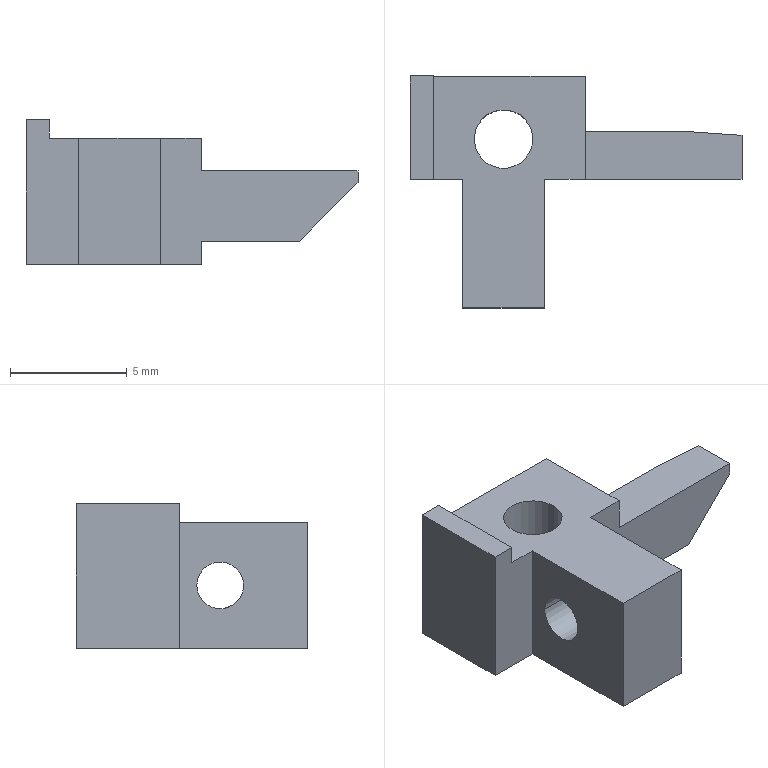Part | NX | 1 solid | 25 faces | box 14.2 x 9.913 x 6.2 mm | volume 267.475 mm3 | plane 19 | cylinder 6 | commonest cylinder face diameters 2 x2 2.5 x2 3.1 x2
STEP:
#1=CARTESIAN_POINT('',(-48.11,-45.316,4.403));
#2=VERTEX_POINT('',#1);
#3=CARTESIAN_POINT('',(-54.61,-45.316,4.403));
#4=VERTEX_POINT('',#3);
#5=CARTESIAN_POINT('',(-49.101,-45.316,4.403));
#6=DIRECTION('',(-1.,0.,0.));
#7=VECTOR('',#6,1000.);
#8=LINE('',#5,#7);
#9=EDGE_CURVE('',#2,#4,#8,.T.);
#10=ORIENTED_EDGE('',*,*,#9,.F.);
#11=CARTESIAN_POINT('',(-48.11,-45.316,-0.9969));
#12=VERTEX_POINT('',#11);
#13=CARTESIAN_POINT('',(-48.11,-45.316,4.403));
#14=DIRECTION('',(0.,0.,-1.));
#15=VECTOR('',#14,1000.);
#16=LINE('',#13,#15);
#17=EDGE_CURVE('',#2,#12,#16,.T.);
#18=ORIENTED_EDGE('',*,*,#17,.T.);
#19=CARTESIAN_POINT('',(-55.61,-45.316,-0.9969));
#20=VERTEX_POINT('',#19);
#21=CARTESIAN_POINT('',(-49.101,-45.316,-0.9969));
#22=DIRECTION('',(-1.,0.,0.));
#23=VECTOR('',#22,1000.);
#24=LINE('',#21,#23);
#25=EDGE_CURVE('',#12,#20,#24,.T.);
#26=ORIENTED_EDGE('',*,*,#25,.T.);
#27=CARTESIAN_POINT('',(-55.61,-45.316,5.203));
#28=VERTEX_POINT('',#27);
#29=CARTESIAN_POINT('',(-55.61,-45.316,4.403));
#30=DIRECTION('',(0.,0.,1.));
#31=VECTOR('',#30,1000.);
#32=LINE('',#29,#31);
#33=EDGE_CURVE('',#20,#28,#32,.T.);
#34=ORIENTED_EDGE('',*,*,#33,.T.);
#35=CARTESIAN_POINT('',(-54.61,-45.316,5.203));
#36=VERTEX_POINT('',#35);
#37=CARTESIAN_POINT('',(-54.61,-45.316,5.203));
#38=DIRECTION('',(-1.,0.,0.));
#39=VECTOR('',#38,1000.);
#40=LINE('',#37,#39);
#41=EDGE_CURVE('',#36,#28,#40,.T.);
#42=ORIENTED_EDGE('',*,*,#41,.F.);
#43=CARTESIAN_POINT('',(-54.61,-45.316,4.403));
#44=DIRECTION('',(0.,0.,1.));
#45=VECTOR('',#44,1000.);
#46=LINE('',#43,#45);
#47=EDGE_CURVE('',#4,#36,#46,.T.);
#48=ORIENTED_EDGE('',*,*,#47,.F.);
#49=EDGE_LOOP('',(#10,#18,#26,#34,#42,#48));
#50=FACE_BOUND('',#49,.T.);
#51=CARTESIAN_POINT('',(-48.11,-45.316,4.403));
#52=DIRECTION('',(0.,1.,0.));
#53=DIRECTION('',(0.,0.,-1.));
#54=AXIS2_PLACEMENT_3D('',#51,#52,#53);
#55=PLANE('',#54);
#56=ADVANCED_FACE('',(#50),#55,.T.);
#57=CARTESIAN_POINT('',(-48.11,-49.729,-0.9969));
#58=VERTEX_POINT('',#57);
#59=CARTESIAN_POINT('',(-48.11,-51.163,-0.9969));
#60=DIRECTION('',(0.,1.,0.));
#61=VECTOR('',#60,1000.);
#62=LINE('',#59,#61);
#63=EDGE_CURVE('',#58,#12,#62,.T.);
#64=ORIENTED_EDGE('',*,*,#63,.F.);
#65=CARTESIAN_POINT('',(-49.86,-49.729,-0.9969));
#66=VERTEX_POINT('',#65);
#67=CARTESIAN_POINT('',(-49.101,-49.729,-0.9969));
#68=DIRECTION('',(-1.,0.,0.));
#69=VECTOR('',#68,1000.);
#70=LINE('',#67,#69);
#71=EDGE_CURVE('',#58,#66,#70,.T.);
#72=ORIENTED_EDGE('',*,*,#71,.T.);
#73=CARTESIAN_POINT('',(-49.86,-55.229,-0.9969));
#74=VERTEX_POINT('',#73);
#75=CARTESIAN_POINT('',(-49.86,-51.163,-0.9969));
#76=DIRECTION('',(0.,-1.,0.));
#77=VECTOR('',#76,1000.);
#78=LINE('',#75,#77);
#79=EDGE_CURVE('',#66,#74,#78,.T.);
#80=ORIENTED_EDGE('',*,*,#79,.T.);
#81=CARTESIAN_POINT('',(-53.36,-55.229,-0.9969));
#82=VERTEX_POINT('',#81);
#83=CARTESIAN_POINT('',(-49.86,-55.229,-0.9969));
#84=DIRECTION('',(-1.,0.,0.));
#85=VECTOR('',#84,1000.);
#86=LINE('',#83,#85);
#87=EDGE_CURVE('',#74,#82,#86,.T.);
#88=ORIENTED_EDGE('',*,*,#87,.T.);
#89=CARTESIAN_POINT('',(-53.36,-49.729,-0.9969));
#90=VERTEX_POINT('',#89);
#91=CARTESIAN_POINT('',(-53.36,-51.163,-0.9969));
#92=DIRECTION('',(0.,-1.,0.));
#93=VECTOR('',#92,1000.);
#94=LINE('',#91,#93);
#95=EDGE_CURVE('',#90,#82,#94,.T.);
#96=ORIENTED_EDGE('',*,*,#95,.F.);
#97=CARTESIAN_POINT('',(-55.61,-49.729,-0.9969));
#98=VERTEX_POINT('',#97);
#99=CARTESIAN_POINT('',(-49.101,-49.729,-0.9969));
#100=DIRECTION('',(-1.,0.,0.));
#101=VECTOR('',#100,1000.);
#102=LINE('',#99,#101);
#103=EDGE_CURVE('',#90,#98,#102,.T.);
#104=ORIENTED_EDGE('',*,*,#103,.T.);
#105=CARTESIAN_POINT('',(-55.61,-51.163,-0.9969));
#106=DIRECTION('',(0.,1.,0.));
#107=VECTOR('',#106,1000.);
#108=LINE('',#105,#107);
#109=EDGE_CURVE('',#98,#20,#108,.T.);
#110=ORIENTED_EDGE('',*,*,#109,.T.);
#111=ORIENTED_EDGE('',*,*,#25,.F.);
#112=EDGE_LOOP('',(#64,#72,#80,#88,#96,#104,#110,#111));
#113=FACE_BOUND('',#112,.T.);
#114=CARTESIAN_POINT('',(-50.36,-48.012,-0.9969));
#115=VERTEX_POINT('',#114);
#116=CARTESIAN_POINT('',(-52.86,-48.012,-0.9969));
#117=VERTEX_POINT('',#116);
#118=CARTESIAN_POINT('',(-51.61,-48.012,-0.9969));
#119=DIRECTION('',(0.,0.,-1.));
#120=DIRECTION('',(-1.,0.,0.));
#121=AXIS2_PLACEMENT_3D('',#118,#119,#120);
#122=CIRCLE('',#121,1.25);
#123=EDGE_CURVE('',#115,#117,#122,.T.);
#124=ORIENTED_EDGE('',*,*,#123,.F.);
#125=CARTESIAN_POINT('',(-51.61,-48.012,-0.9969));
#126=DIRECTION('',(0.,0.,-1.));
#127=DIRECTION('',(-1.,0.,0.));
#128=AXIS2_PLACEMENT_3D('',#125,#126,#127);
#129=CIRCLE('',#128,1.25);
#130=EDGE_CURVE('',#117,#115,#129,.T.);
#131=ORIENTED_EDGE('',*,*,#130,.F.);
#132=EDGE_LOOP('',(#124,#131));
#133=FACE_BOUND('',#132,.T.);
#134=CARTESIAN_POINT('',(-50.06,-53.51,-0.9969));
#135=VERTEX_POINT('',#134);
#136=CARTESIAN_POINT('',(-53.16,-53.51,-0.9969));
#137=VERTEX_POINT('',#136);
#138=CARTESIAN_POINT('',(-51.61,-53.51,-0.9969));
#139=DIRECTION('',(0.,0.,-1.));
#140=DIRECTION('',(-1.,0.,0.));
#141=AXIS2_PLACEMENT_3D('',#138,#139,#140);
#142=CIRCLE('',#141,1.55);
#143=EDGE_CURVE('',#135,#137,#142,.T.);
#144=ORIENTED_EDGE('',*,*,#143,.F.);
#145=CARTESIAN_POINT('',(-51.61,-53.51,-0.9969));
#146=DIRECTION('',(0.,0.,-1.));
#147=DIRECTION('',(-1.,0.,0.));
#148=AXIS2_PLACEMENT_3D('',#145,#146,#147);
#149=CIRCLE('',#148,1.55);
#150=EDGE_CURVE('',#137,#135,#149,.T.);
#151=ORIENTED_EDGE('',*,*,#150,.F.);
#152=EDGE_LOOP('',(#144,#151));
#153=FACE_BOUND('',#152,.T.);
#154=CARTESIAN_POINT('',(-49.101,-51.163,-0.9969));
#155=DIRECTION('',(0.,0.,-1.));
#156=DIRECTION('',(0.,-1.,0.));
#157=AXIS2_PLACEMENT_3D('',#154,#155,#156);
#158=PLANE('',#157);
#159=ADVANCED_FACE('',(#113,#133,#153),#158,.T.);
#160=ORIENTED_EDGE('',*,*,#63,.T.);
#161=ORIENTED_EDGE('',*,*,#17,.F.);
#162=CARTESIAN_POINT('',(-48.11,-49.729,4.403));
#163=VERTEX_POINT('',#162);
#164=CARTESIAN_POINT('',(-48.11,-51.163,4.403));
#165=DIRECTION('',(0.,1.,0.));
#166=VECTOR('',#165,1000.);
#167=LINE('',#164,#166);
#168=EDGE_CURVE('',#163,#2,#167,.T.);
#169=ORIENTED_EDGE('',*,*,#168,.F.);
#170=CARTESIAN_POINT('',(-48.11,-49.729,3.003));
#171=VERTEX_POINT('',#170);
#172=CARTESIAN_POINT('',(-48.11,-49.729,4.403));
#173=DIRECTION('',(0.,0.,-1.));
#174=VECTOR('',#173,1000.);
#175=LINE('',#172,#174);
#176=EDGE_CURVE('',#163,#171,#175,.T.);
#177=ORIENTED_EDGE('',*,*,#176,.T.);
#178=CARTESIAN_POINT('',(-48.11,-47.687,3.003));
#179=VERTEX_POINT('',#178);
#180=CARTESIAN_POINT('',(-48.11,-51.163,3.003));
#181=DIRECTION('',(0.,-1.,0.));
#182=VECTOR('',#181,1000.);
#183=LINE('',#180,#182);
#184=EDGE_CURVE('',#179,#171,#183,.T.);
#185=ORIENTED_EDGE('',*,*,#184,.F.);
#186=CARTESIAN_POINT('',(-48.11,-47.687,0.003122));
#187=VERTEX_POINT('',#186);
#188=CARTESIAN_POINT('',(-48.11,-47.687,4.403));
#189=DIRECTION('',(0.,0.,1.));
#190=VECTOR('',#189,1000.);
#191=LINE('',#188,#190);
#192=EDGE_CURVE('',#187,#179,#191,.T.);
#193=ORIENTED_EDGE('',*,*,#192,.F.);
#194=CARTESIAN_POINT('',(-48.11,-49.729,0.003122));
#195=VERTEX_POINT('',#194);
#196=CARTESIAN_POINT('',(-48.11,-51.163,0.003122));
#197=DIRECTION('',(0.,1.,0.));
#198=VECTOR('',#197,1000.);
#199=LINE('',#196,#198);
#200=EDGE_CURVE('',#195,#187,#199,.T.);
#201=ORIENTED_EDGE('',*,*,#200,.F.);
#202=CARTESIAN_POINT('',(-48.11,-49.729,4.403));
#203=DIRECTION('',(0.,0.,-1.));
#204=VECTOR('',#203,1000.);
#205=LINE('',#202,#204);
#206=EDGE_CURVE('',#195,#58,#205,.T.);
#207=ORIENTED_EDGE('',*,*,#206,.T.);
#208=EDGE_LOOP('',(#160,#161,#169,#177,#185,#193,#201,#207));
#209=FACE_BOUND('',#208,.T.);
#210=CARTESIAN_POINT('',(-48.11,-47.529,-0.5969));
#211=DIRECTION('',(1.,0.,0.));
#212=DIRECTION('',(0.,1.,0.));
#213=AXIS2_PLACEMENT_3D('',#210,#211,#212);
#214=PLANE('',#213);
#215=ADVANCED_FACE('',(#209),#214,.T.);
#216=CARTESIAN_POINT('',(-55.61,-49.729,5.203));
#217=VERTEX_POINT('',#216);
#218=CARTESIAN_POINT('',(-55.61,-45.316,5.203));
#219=DIRECTION('',(0.,-1.,0.));
#220=VECTOR('',#219,1000.);
#221=LINE('',#218,#220);
#222=EDGE_CURVE('',#28,#217,#221,.T.);
#223=ORIENTED_EDGE('',*,*,#222,.T.);
#224=CARTESIAN_POINT('',(-54.61,-49.729,5.203));
#225=VERTEX_POINT('',#224);
#226=CARTESIAN_POINT('',(-55.61,-49.729,5.203));
#227=DIRECTION('',(1.,0.,0.));
#228=VECTOR('',#227,1000.);
#229=LINE('',#226,#228);
#230=EDGE_CURVE('',#217,#225,#229,.T.);
#231=ORIENTED_EDGE('',*,*,#230,.T.);
#232=CARTESIAN_POINT('',(-54.61,-49.729,5.203));
#233=DIRECTION('',(0.,1.,0.));
#234=VECTOR('',#233,1000.);
#235=LINE('',#232,#234);
#236=EDGE_CURVE('',#225,#36,#235,.T.);
#237=ORIENTED_EDGE('',*,*,#236,.T.);
#238=ORIENTED_EDGE('',*,*,#41,.T.);
#239=EDGE_LOOP('',(#223,#231,#237,#238));
#240=FACE_BOUND('',#239,.T.);
#241=CARTESIAN_POINT('',(-55.143,-49.311,5.203));
#242=DIRECTION('',(0.,0.,1.));
#243=DIRECTION('',(1.,0.,0.));
#244=AXIS2_PLACEMENT_3D('',#241,#242,#243);
#245=PLANE('',#244);
#246=ADVANCED_FACE('',(#240),#245,.T.);
#247=CARTESIAN_POINT('',(-55.61,-49.729,4.403));
#248=DIRECTION('',(0.,0.,-1.));
#249=VECTOR('',#248,1000.);
#250=LINE('',#247,#249);
#251=EDGE_CURVE('',#217,#98,#250,.T.);
#252=ORIENTED_EDGE('',*,*,#251,.F.);
#253=ORIENTED_EDGE('',*,*,#222,.F.);
#254=ORIENTED_EDGE('',*,*,#33,.F.);
#255=ORIENTED_EDGE('',*,*,#109,.F.);
#256=EDGE_LOOP('',(#252,#253,#254,#255));
#257=FACE_BOUND('',#256,.T.);
#258=CARTESIAN_POINT('',(-55.61,-49.729,4.403));
#259=DIRECTION('',(-1.,0.,0.));
#260=DIRECTION('',(0.,0.,1.));
#261=AXIS2_PLACEMENT_3D('',#258,#259,#260);
#262=PLANE('',#261);
#263=ADVANCED_FACE('',(#257),#262,.T.);
#264=CARTESIAN_POINT('',(-54.61,-49.729,4.403));
#265=VERTEX_POINT('',#264);
#266=CARTESIAN_POINT('',(-54.61,-51.163,4.403));
#267=DIRECTION('',(0.,-1.,0.));
#268=VECTOR('',#267,1000.);
#269=LINE('',#266,#268);
#270=EDGE_CURVE('',#4,#265,#269,.T.);
#271=ORIENTED_EDGE('',*,*,#270,.F.);
#272=ORIENTED_EDGE('',*,*,#47,.T.);
#273=ORIENTED_EDGE('',*,*,#236,.F.);
#274=CARTESIAN_POINT('',(-54.61,-49.729,4.403));
#275=DIRECTION('',(0.,0.,1.));
#276=VECTOR('',#275,1000.);
#277=LINE('',#274,#276);
#278=EDGE_CURVE('',#265,#225,#277,.T.);
#279=ORIENTED_EDGE('',*,*,#278,.F.);
#280=EDGE_LOOP('',(#271,#272,#273,#279));
#281=FACE_BOUND('',#280,.T.);
#282=CARTESIAN_POINT('',(-54.61,-45.316,4.403));
#283=DIRECTION('',(1.,0.,0.));
#284=DIRECTION('',(0.,1.,0.));
#285=AXIS2_PLACEMENT_3D('',#282,#283,#284);
#286=PLANE('',#285);
#287=ADVANCED_FACE('',(#281),#286,.T.);
#288=ORIENTED_EDGE('',*,*,#278,.T.);
#289=ORIENTED_EDGE('',*,*,#230,.F.);
#290=ORIENTED_EDGE('',*,*,#251,.T.);
#291=ORIENTED_EDGE('',*,*,#103,.F.);
#292=CARTESIAN_POINT('',(-53.36,-49.729,4.403));
#293=VERTEX_POINT('',#292);
#294=CARTESIAN_POINT('',(-53.36,-49.729,4.403));
#295=DIRECTION('',(0.,0.,1.));
#296=VECTOR('',#295,1000.);
#297=LINE('',#294,#296);
#298=EDGE_CURVE('',#90,#293,#297,.T.);
#299=ORIENTED_EDGE('',*,*,#298,.T.);
#300=CARTESIAN_POINT('',(-49.101,-49.729,4.403));
#301=DIRECTION('',(1.,0.,0.));
#302=VECTOR('',#301,1000.);
#303=LINE('',#300,#302);
#304=EDGE_CURVE('',#265,#293,#303,.T.);
#305=ORIENTED_EDGE('',*,*,#304,.F.);
#306=EDGE_LOOP('',(#288,#289,#290,#291,#299,#305));
#307=FACE_BOUND('',#306,.T.);
#308=CARTESIAN_POINT('',(-54.61,-49.729,4.403));
#309=DIRECTION('',(0.,-1.,0.));
#310=DIRECTION('',(0.,0.,-1.));
#311=AXIS2_PLACEMENT_3D('',#308,#309,#310);
#312=PLANE('',#311);
#313=ADVANCED_FACE('',(#307),#312,.T.);
#314=CARTESIAN_POINT('',(-43.739,-47.687,3.003));
#315=VERTEX_POINT('',#314);
#316=CARTESIAN_POINT('',(-49.101,-47.687,3.003));
#317=DIRECTION('',(1.,0.,0.));
#318=VECTOR('',#317,1000.);
#319=LINE('',#316,#318);
#320=EDGE_CURVE('',#179,#315,#319,.T.);
#321=ORIENTED_EDGE('',*,*,#320,.F.);
#322=ORIENTED_EDGE('',*,*,#184,.T.);
#323=CARTESIAN_POINT('',(-41.41,-49.729,3.003));
#324=VERTEX_POINT('',#323);
#325=CARTESIAN_POINT('',(-49.101,-49.729,3.003));
#326=DIRECTION('',(1.,0.,0.));
#327=VECTOR('',#326,1000.);
#328=LINE('',#325,#327);
#329=EDGE_CURVE('',#171,#324,#328,.T.);
#330=ORIENTED_EDGE('',*,*,#329,.T.);
#331=CARTESIAN_POINT('',(-41.41,-47.851,3.003));
#332=VERTEX_POINT('',#331);
#333=CARTESIAN_POINT('',(-41.41,-51.163,3.003));
#334=DIRECTION('',(0.,1.,0.));
#335=VECTOR('',#334,1000.);
#336=LINE('',#333,#335);
#337=EDGE_CURVE('',#324,#332,#336,.T.);
#338=ORIENTED_EDGE('',*,*,#337,.T.);
#339=CARTESIAN_POINT('',(-49.101,-47.307,3.003));
#340=DIRECTION('',(0.9975,-0.07053,0.));
#341=VECTOR('',#340,1000.);
#342=LINE('',#339,#341);
#343=EDGE_CURVE('',#315,#332,#342,.T.);
#344=ORIENTED_EDGE('',*,*,#343,.F.);
#345=EDGE_LOOP('',(#321,#322,#330,#338,#344));
#346=FACE_BOUND('',#345,.T.);
#347=CARTESIAN_POINT('',(-48.11,-53.629,3.003));
#348=DIRECTION('',(0.,0.,1.));
#349=DIRECTION('',(1.,0.,0.));
#350=AXIS2_PLACEMENT_3D('',#347,#348,#349);
#351=PLANE('',#350);
#352=ADVANCED_FACE('',(#346),#351,.T.);
#353=ORIENTED_EDGE('',*,*,#123,.T.);
#354=CARTESIAN_POINT('',(-52.86,-48.012,4.403));
#355=VERTEX_POINT('',#354);
#356=CARTESIAN_POINT('',(-52.86,-48.012,-2.597));
#357=DIRECTION('',(0.,0.,-1.));
#358=VECTOR('',#357,1000.);
#359=LINE('',#356,#358);
#360=EDGE_CURVE('',#117,#355,#359,.F.);
#361=ORIENTED_EDGE('',*,*,#360,.T.);
#362=CARTESIAN_POINT('',(-50.36,-48.012,4.403));
#363=VERTEX_POINT('',#362);
#364=CARTESIAN_POINT('',(-51.61,-48.012,4.403));
#365=DIRECTION('',(0.,0.,-1.));
#366=DIRECTION('',(-1.,0.,0.));
#367=AXIS2_PLACEMENT_3D('',#364,#365,#366);
#368=CIRCLE('',#367,1.25);
#369=EDGE_CURVE('',#363,#355,#368,.T.);
#370=ORIENTED_EDGE('',*,*,#369,.F.);
#371=CARTESIAN_POINT('',(-50.36,-48.012,-2.597));
#372=DIRECTION('',(0.,0.,-1.));
#373=VECTOR('',#372,1000.);
#374=LINE('',#371,#373);
#375=EDGE_CURVE('',#115,#363,#374,.F.);
#376=ORIENTED_EDGE('',*,*,#375,.F.);
#377=EDGE_LOOP('',(#353,#361,#370,#376));
#378=FACE_BOUND('',#377,.T.);
#379=CARTESIAN_POINT('',(-51.61,-48.012,-2.597));
#380=DIRECTION('',(0.,0.,-1.));
#381=DIRECTION('',(-1.,0.,0.));
#382=AXIS2_PLACEMENT_3D('',#379,#380,#381);
#383=CYLINDRICAL_SURFACE('',#382,1.25);
#384=ADVANCED_FACE('',(#378),#383,.F.);
#385=ORIENTED_EDGE('',*,*,#320,.T.);
#386=CARTESIAN_POINT('',(-46.739,-47.687,0.003122));
#387=VERTEX_POINT('',#386);
#388=CARTESIAN_POINT('',(-44.574,-47.687,2.167));
#389=DIRECTION('',(0.7071,0.,0.7071));
#390=VECTOR('',#389,1000.);
#391=LINE('',#388,#390);
#392=EDGE_CURVE('',#387,#315,#391,.T.);
#393=ORIENTED_EDGE('',*,*,#392,.F.);
#394=CARTESIAN_POINT('',(-49.101,-47.687,0.003122));
#395=DIRECTION('',(-1.,0.,0.));
#396=VECTOR('',#395,1000.);
#397=LINE('',#394,#396);
#398=EDGE_CURVE('',#387,#187,#397,.T.);
#399=ORIENTED_EDGE('',*,*,#398,.T.);
#400=ORIENTED_EDGE('',*,*,#192,.T.);
#401=EDGE_LOOP('',(#385,#393,#399,#400));
#402=FACE_BOUND('',#401,.T.);
#403=CARTESIAN_POINT('',(-48.11,-47.687,2.503));
#404=DIRECTION('',(0.,1.,0.));
#405=DIRECTION('',(1.,0.,0.));
#406=AXIS2_PLACEMENT_3D('',#403,#404,#405);
#407=PLANE('',#406);
#408=ADVANCED_FACE('',(#402),#407,.T.);
#409=ORIENTED_EDGE('',*,*,#143,.T.);
#410=CARTESIAN_POINT('',(-53.16,-53.51,1.003));
#411=VERTEX_POINT('',#410);
#412=CARTESIAN_POINT('',(-53.16,-53.51,-0.9969));
#413=DIRECTION('',(0.,0.,-1.));
#414=VECTOR('',#413,1000.);
#415=LINE('',#412,#414);
#416=EDGE_CURVE('',#137,#411,#415,.F.);
#417=ORIENTED_EDGE('',*,*,#416,.T.);
#418=CARTESIAN_POINT('',(-50.06,-53.51,1.003));
#419=VERTEX_POINT('',#418);
#420=CARTESIAN_POINT('',(-51.61,-53.51,1.003));
#421=DIRECTION('',(0.,0.,-1.));
#422=DIRECTION('',(-1.,0.,0.));
#423=AXIS2_PLACEMENT_3D('',#420,#421,#422);
#424=CIRCLE('',#423,1.55);
#425=EDGE_CURVE('',#419,#411,#424,.T.);
#426=ORIENTED_EDGE('',*,*,#425,.F.);
#427=CARTESIAN_POINT('',(-50.06,-53.51,-0.9969));
#428=DIRECTION('',(0.,0.,-1.));
#429=VECTOR('',#428,1000.);
#430=LINE('',#427,#429);
#431=EDGE_CURVE('',#135,#419,#430,.F.);
#432=ORIENTED_EDGE('',*,*,#431,.F.);
#433=EDGE_LOOP('',(#409,#417,#426,#432));
#434=FACE_BOUND('',#433,.T.);
#435=CARTESIAN_POINT('',(-51.61,-53.51,-0.9969));
#436=DIRECTION('',(0.,0.,-1.));
#437=DIRECTION('',(-1.,0.,0.));
#438=AXIS2_PLACEMENT_3D('',#435,#436,#437);
#439=CYLINDRICAL_SURFACE('',#438,1.55);
#440=ADVANCED_FACE('',(#434),#439,.F.);
#441=CARTESIAN_POINT('',(-41.41,-49.729,2.503));
#442=VERTEX_POINT('',#441);
#443=CARTESIAN_POINT('',(-41.41,-47.887,2.503));
#444=VERTEX_POINT('',#443);
#445=CARTESIAN_POINT('',(-41.41,-51.163,2.503));
#446=DIRECTION('',(0.,1.,0.));
#447=VECTOR('',#446,1000.);
#448=LINE('',#445,#447);
#449=EDGE_CURVE('',#442,#444,#448,.T.);
#450=ORIENTED_EDGE('',*,*,#449,.T.);
#451=CARTESIAN_POINT('',(-41.41,-47.752,4.403));
#452=DIRECTION('',(0.,-0.07053,-0.9975));
#453=VECTOR('',#452,1000.);
#454=LINE('',#451,#453);
#455=EDGE_CURVE('',#332,#444,#454,.T.);
#456=ORIENTED_EDGE('',*,*,#455,.F.);
#457=ORIENTED_EDGE('',*,*,#337,.F.);
#458=CARTESIAN_POINT('',(-41.41,-49.729,4.403));
#459=DIRECTION('',(0.,0.,-1.));
#460=VECTOR('',#459,1000.);
#461=LINE('',#458,#460);
#462=EDGE_CURVE('',#324,#442,#461,.T.);
#463=ORIENTED_EDGE('',*,*,#462,.T.);
#464=EDGE_LOOP('',(#450,#456,#457,#463));
#465=FACE_BOUND('',#464,.T.);
#466=CARTESIAN_POINT('',(-41.41,-49.37,2.047));
#467=DIRECTION('',(1.,0.,0.));
#468=DIRECTION('',(0.,1.,0.));
#469=AXIS2_PLACEMENT_3D('',#466,#467,#468);
#470=PLANE('',#469);
#471=ADVANCED_FACE('',(#465),#470,.T.);
#472=CARTESIAN_POINT('',(-43.91,-47.887,0.003122));
#473=VERTEX_POINT('',#472);
#474=CARTESIAN_POINT('',(-43.16,-47.887,0.7531));
#475=DIRECTION('',(0.7071,0.,0.7071));
#476=VECTOR('',#475,1000.);
#477=LINE('',#474,#476);
#478=EDGE_CURVE('',#473,#444,#477,.T.);
#479=ORIENTED_EDGE('',*,*,#478,.T.);
#480=ORIENTED_EDGE('',*,*,#449,.F.);
#481=CARTESIAN_POINT('',(-43.91,-49.729,0.003122));
#482=VERTEX_POINT('',#481);
#483=CARTESIAN_POINT('',(-39.51,-49.729,4.403));
#484=DIRECTION('',(-0.7071,0.,-0.7071));
#485=VECTOR('',#484,1000.);
#486=LINE('',#483,#485);
#487=EDGE_CURVE('',#442,#482,#486,.T.);
#488=ORIENTED_EDGE('',*,*,#487,.T.);
#489=CARTESIAN_POINT('',(-43.91,-51.163,0.003122));
#490=DIRECTION('',(0.,1.,0.));
#491=VECTOR('',#490,1000.);
#492=LINE('',#489,#491);
#493=EDGE_CURVE('',#482,#473,#492,.T.);
#494=ORIENTED_EDGE('',*,*,#493,.T.);
#495=EDGE_LOOP('',(#479,#480,#488,#494));
#496=FACE_BOUND('',#495,.T.);
#497=CARTESIAN_POINT('',(-43.16,-50.658,0.7531));
#498=DIRECTION('',(0.7071,0.,-0.7071));
#499=DIRECTION('',(0.,-1.,0.));
#500=AXIS2_PLACEMENT_3D('',#497,#498,#499);
#501=PLANE('',#500);
#502=ADVANCED_FACE('',(#496),#501,.T.);
#503=ORIENTED_EDGE('',*,*,#478,.F.);
#504=CARTESIAN_POINT('',(-49.101,-47.52,0.003122));
#505=DIRECTION('',(-0.9975,0.07053,0.));
#506=VECTOR('',#505,1000.);
#507=LINE('',#504,#506);
#508=EDGE_CURVE('',#473,#387,#507,.T.);
#509=ORIENTED_EDGE('',*,*,#508,.T.);
#510=ORIENTED_EDGE('',*,*,#392,.T.);
#511=ORIENTED_EDGE('',*,*,#343,.T.);
#512=ORIENTED_EDGE('',*,*,#455,.T.);
#513=EDGE_LOOP('',(#503,#509,#510,#511,#512));
#514=FACE_BOUND('',#513,.T.);
#515=CARTESIAN_POINT('',(-43.867,-47.787,1.46));
#516=DIRECTION('',(0.07036,0.995,-0.07036));
#517=DIRECTION('',(-0.7071,0.,-0.7071));
#518=AXIS2_PLACEMENT_3D('',#515,#516,#517);
#519=PLANE('',#518);
#520=ADVANCED_FACE('',(#514),#519,.T.);
#521=CARTESIAN_POINT('',(-49.101,-49.729,0.003122));
#522=DIRECTION('',(-1.,0.,0.));
#523=VECTOR('',#522,1000.);
#524=LINE('',#521,#523);
#525=EDGE_CURVE('',#482,#195,#524,.T.);
#526=ORIENTED_EDGE('',*,*,#525,.T.);
#527=ORIENTED_EDGE('',*,*,#200,.T.);
#528=ORIENTED_EDGE('',*,*,#398,.F.);
#529=ORIENTED_EDGE('',*,*,#508,.F.);
#530=ORIENTED_EDGE('',*,*,#493,.F.);
#531=EDGE_LOOP('',(#526,#527,#528,#529,#530));
#532=FACE_BOUND('',#531,.T.);
#533=CARTESIAN_POINT('',(-46.061,-49.047,0.003122));
#534=DIRECTION('',(0.,0.,-1.));
#535=DIRECTION('',(0.,-1.,0.));
#536=AXIS2_PLACEMENT_3D('',#533,#534,#535);
#537=PLANE('',#536);
#538=ADVANCED_FACE('',(#532),#537,.T.);
#539=CARTESIAN_POINT('',(-49.86,-49.729,4.403));
#540=VERTEX_POINT('',#539);
#541=CARTESIAN_POINT('',(-49.86,-49.729,4.403));
#542=DIRECTION('',(0.,0.,-1.));
#543=VECTOR('',#542,1000.);
#544=LINE('',#541,#543);
#545=EDGE_CURVE('',#540,#66,#544,.T.);
#546=ORIENTED_EDGE('',*,*,#545,.T.);
#547=ORIENTED_EDGE('',*,*,#71,.F.);
#548=ORIENTED_EDGE('',*,*,#206,.F.);
#549=ORIENTED_EDGE('',*,*,#525,.F.);
#550=ORIENTED_EDGE('',*,*,#487,.F.);
#551=ORIENTED_EDGE('',*,*,#462,.F.);
#552=ORIENTED_EDGE('',*,*,#329,.F.);
#553=ORIENTED_EDGE('',*,*,#176,.F.);
#554=CARTESIAN_POINT('',(-49.101,-49.729,4.403));
#555=DIRECTION('',(1.,0.,0.));
#556=VECTOR('',#555,1000.);
#557=LINE('',#554,#556);
#558=EDGE_CURVE('',#540,#163,#557,.T.);
#559=ORIENTED_EDGE('',*,*,#558,.F.);
#560=EDGE_LOOP('',(#546,#547,#548,#549,#550,#551,#552,#553,#559));
#561=FACE_BOUND('',#560,.T.);
#562=CARTESIAN_POINT('',(-48.11,-49.729,-0.5969));
#563=DIRECTION('',(0.,-1.,0.));
#564=DIRECTION('',(0.,0.,-1.));
#565=AXIS2_PLACEMENT_3D('',#562,#563,#564);
#566=PLANE('',#565);
#567=ADVANCED_FACE('',(#561),#566,.T.);
#568=ORIENTED_EDGE('',*,*,#298,.F.);
#569=ORIENTED_EDGE('',*,*,#95,.T.);
#570=CARTESIAN_POINT('',(-53.36,-55.229,4.403));
#571=VERTEX_POINT('',#570);
#572=CARTESIAN_POINT('',(-53.36,-55.229,4.403));
#573=DIRECTION('',(0.,0.,1.));
#574=VECTOR('',#573,1000.);
#575=LINE('',#572,#574);
#576=EDGE_CURVE('',#82,#571,#575,.T.);
#577=ORIENTED_EDGE('',*,*,#576,.T.);
#578=CARTESIAN_POINT('',(-53.36,-51.163,4.403));
#579=DIRECTION('',(0.,-1.,0.));
#580=VECTOR('',#579,1000.);
#581=LINE('',#578,#580);
#582=EDGE_CURVE('',#293,#571,#581,.T.);
#583=ORIENTED_EDGE('',*,*,#582,.F.);
#584=EDGE_LOOP('',(#568,#569,#577,#583));
#585=FACE_BOUND('',#584,.T.);
#586=CARTESIAN_POINT('',(-53.36,-50.479,1.703));
#587=VERTEX_POINT('',#586);
#588=CARTESIAN_POINT('',(-53.36,-52.479,1.703));
#589=VERTEX_POINT('',#588);
#590=CARTESIAN_POINT('',(-53.36,-51.479,1.703));
#591=DIRECTION('',(-1.,0.,0.));
#592=DIRECTION('',(0.,-1.,0.));
#593=AXIS2_PLACEMENT_3D('',#590,#591,#592);
#594=CIRCLE('',#593,1.);
#595=EDGE_CURVE('',#587,#589,#594,.T.);
#596=ORIENTED_EDGE('',*,*,#595,.F.);
#597=CARTESIAN_POINT('',(-53.36,-51.479,1.703));
#598=DIRECTION('',(-1.,0.,0.));
#599=DIRECTION('',(0.,-1.,0.));
#600=AXIS2_PLACEMENT_3D('',#597,#598,#599);
#601=CIRCLE('',#600,1.);
#602=EDGE_CURVE('',#589,#587,#601,.T.);
#603=ORIENTED_EDGE('',*,*,#602,.F.);
#604=EDGE_LOOP('',(#596,#603));
#605=FACE_BOUND('',#604,.T.);
#606=CARTESIAN_POINT('',(-53.36,-50.229,-0.9969));
#607=DIRECTION('',(-1.,0.,0.));
#608=DIRECTION('',(0.,0.,1.));
#609=AXIS2_PLACEMENT_3D('',#606,#607,#608);
#610=PLANE('',#609);
#611=ADVANCED_FACE('',(#585,#605),#610,.T.);
#612=ORIENTED_EDGE('',*,*,#545,.F.);
#613=CARTESIAN_POINT('',(-49.86,-55.229,4.403));
#614=VERTEX_POINT('',#613);
#615=CARTESIAN_POINT('',(-49.86,-51.163,4.403));
#616=DIRECTION('',(0.,1.,0.));
#617=VECTOR('',#616,1000.);
#618=LINE('',#615,#617);
#619=EDGE_CURVE('',#614,#540,#618,.T.);
#620=ORIENTED_EDGE('',*,*,#619,.F.);
#621=CARTESIAN_POINT('',(-49.86,-55.229,4.403));
#622=DIRECTION('',(0.,0.,-1.));
#623=VECTOR('',#622,1000.);
#624=LINE('',#621,#623);
#625=EDGE_CURVE('',#614,#74,#624,.T.);
#626=ORIENTED_EDGE('',*,*,#625,.T.);
#627=ORIENTED_EDGE('',*,*,#79,.F.);
#628=EDGE_LOOP('',(#612,#620,#626,#627));
#629=FACE_BOUND('',#628,.T.);
#630=CARTESIAN_POINT('',(-49.86,-50.479,1.703));
#631=VERTEX_POINT('',#630);
#632=CARTESIAN_POINT('',(-49.86,-52.479,1.703));
#633=VERTEX_POINT('',#632);
#634=CARTESIAN_POINT('',(-49.86,-51.479,1.703));
#635=DIRECTION('',(-1.,0.,0.));
#636=DIRECTION('',(0.,-1.,0.));
#637=AXIS2_PLACEMENT_3D('',#634,#635,#636);
#638=CIRCLE('',#637,1.);
#639=EDGE_CURVE('',#631,#633,#638,.T.);
#640=ORIENTED_EDGE('',*,*,#639,.T.);
#641=CARTESIAN_POINT('',(-49.86,-51.479,1.703));
#642=DIRECTION('',(-1.,0.,0.));
#643=DIRECTION('',(0.,-1.,0.));
#644=AXIS2_PLACEMENT_3D('',#641,#642,#643);
#645=CIRCLE('',#644,1.);
#646=EDGE_CURVE('',#633,#631,#645,.T.);
#647=ORIENTED_EDGE('',*,*,#646,.T.);
#648=EDGE_LOOP('',(#640,#647));
#649=FACE_BOUND('',#648,.T.);
#650=CARTESIAN_POINT('',(-49.86,-50.229,4.403));
#651=DIRECTION('',(1.,0.,0.));
#652=DIRECTION('',(0.,1.,0.));
#653=AXIS2_PLACEMENT_3D('',#650,#651,#652);
#654=PLANE('',#653);
#655=ADVANCED_FACE('',(#629,#649),#654,.T.);
#656=ORIENTED_EDGE('',*,*,#576,.F.);
#657=ORIENTED_EDGE('',*,*,#87,.F.);
#658=ORIENTED_EDGE('',*,*,#625,.F.);
#659=CARTESIAN_POINT('',(-49.101,-55.229,4.403));
#660=DIRECTION('',(1.,0.,0.));
#661=VECTOR('',#660,1000.);
#662=LINE('',#659,#661);
#663=EDGE_CURVE('',#571,#614,#662,.T.);
#664=ORIENTED_EDGE('',*,*,#663,.F.);
#665=EDGE_LOOP('',(#656,#657,#658,#664));
#666=FACE_BOUND('',#665,.T.);
#667=CARTESIAN_POINT('',(-51.674,-55.229,-0.05073));
#668=DIRECTION('',(0.,-1.,0.));
#669=DIRECTION('',(0.,0.,-1.));
#670=AXIS2_PLACEMENT_3D('',#667,#668,#669);
#671=PLANE('',#670);
#672=ADVANCED_FACE('',(#666),#671,.T.);
#673=ORIENTED_EDGE('',*,*,#639,.F.);
#674=CARTESIAN_POINT('',(-40.04,-50.479,1.703));
#675=DIRECTION('',(-1.,0.,0.));
#676=VECTOR('',#675,1000.);
#677=LINE('',#674,#676);
#678=EDGE_CURVE('',#587,#631,#677,.F.);
#679=ORIENTED_EDGE('',*,*,#678,.F.);
#680=ORIENTED_EDGE('',*,*,#595,.T.);
#681=CARTESIAN_POINT('',(-40.04,-52.479,1.703));
#682=DIRECTION('',(-1.,0.,0.));
#683=VECTOR('',#682,1000.);
#684=LINE('',#681,#683);
#685=EDGE_CURVE('',#589,#633,#684,.F.);
#686=ORIENTED_EDGE('',*,*,#685,.T.);
#687=EDGE_LOOP('',(#673,#679,#680,#686));
#688=FACE_BOUND('',#687,.T.);
#689=CARTESIAN_POINT('',(-52.427,-52.193,1.003));
#690=VERTEX_POINT('',#689);
#691=CARTESIAN_POINT('',(-50.793,-52.193,1.003));
#692=VERTEX_POINT('',#691);
#693=CARTESIAN_POINT('',(-52.427,-52.193,1.003));
#694=CARTESIAN_POINT('',(-52.414,-52.185,0.9943));
#695=CARTESIAN_POINT('',(-52.399,-52.176,0.986));
#696=CARTESIAN_POINT('',(-52.385,-52.168,0.9781));
#697=CARTESIAN_POINT('',(-52.37,-52.159,0.9701));
#698=CARTESIAN_POINT('',(-52.356,-52.151,0.9626));
#699=CARTESIAN_POINT('',(-52.341,-52.143,0.9555));
#700=CARTESIAN_POINT('',(-52.326,-52.135,0.9484));
#701=CARTESIAN_POINT('',(-52.311,-52.127,0.9417));
#702=CARTESIAN_POINT('',(-52.295,-52.12,0.9353));
#703=CARTESIAN_POINT('',(-52.28,-52.112,0.929));
#704=CARTESIAN_POINT('',(-52.264,-52.105,0.923));
#705=CARTESIAN_POINT('',(-52.248,-52.097,0.9173));
#706=CARTESIAN_POINT('',(-52.232,-52.09,0.9116));
#707=CARTESIAN_POINT('',(-52.215,-52.083,0.9062));
#708=CARTESIAN_POINT('',(-52.199,-52.076,0.9012));
#709=CARTESIAN_POINT('',(-52.183,-52.07,0.8962));
#710=CARTESIAN_POINT('',(-52.166,-52.063,0.8914));
#711=CARTESIAN_POINT('',(-52.149,-52.057,0.887));
#712=CARTESIAN_POINT('',(-52.132,-52.051,0.8826));
#713=CARTESIAN_POINT('',(-52.115,-52.045,0.8785));
#714=CARTESIAN_POINT('',(-52.098,-52.039,0.8746));
#715=CARTESIAN_POINT('',(-52.081,-52.033,0.8708));
#716=CARTESIAN_POINT('',(-52.063,-52.028,0.8672));
#717=CARTESIAN_POINT('',(-52.046,-52.023,0.8639));
#718=CARTESIAN_POINT('',(-52.029,-52.018,0.8606));
#719=CARTESIAN_POINT('',(-52.011,-52.013,0.8575));
#720=CARTESIAN_POINT('',(-51.993,-52.008,0.8547));
#721=CARTESIAN_POINT('',(-51.976,-52.004,0.8519));
#722=CARTESIAN_POINT('',(-51.958,-52.,0.8494));
#723=CARTESIAN_POINT('',(-51.94,-51.996,0.847));
#724=CARTESIAN_POINT('',(-51.905,-51.988,0.8423));
#725=CARTESIAN_POINT('',(-51.868,-51.981,0.8385));
#726=CARTESIAN_POINT('',(-51.832,-51.976,0.8355));
#727=CARTESIAN_POINT('',(-51.795,-51.971,0.8324));
#728=CARTESIAN_POINT('',(-51.758,-51.967,0.8302));
#729=CARTESIAN_POINT('',(-51.721,-51.964,0.8287));
#730=CARTESIAN_POINT('',(-51.685,-51.962,0.8273));
#731=CARTESIAN_POINT('',(-51.647,-51.96,0.8265));
#732=CARTESIAN_POINT('',(-51.61,-51.96,0.8265));
#733=CARTESIAN_POINT('',(-51.573,-51.96,0.8265));
#734=CARTESIAN_POINT('',(-51.536,-51.962,0.8273));
#735=CARTESIAN_POINT('',(-51.5,-51.964,0.8287));
#736=CARTESIAN_POINT('',(-51.481,-51.965,0.8294));
#737=CARTESIAN_POINT('',(-51.463,-51.967,0.8304));
#738=CARTESIAN_POINT('',(-51.445,-51.969,0.8315));
#739=CARTESIAN_POINT('',(-51.427,-51.971,0.8326));
#740=CARTESIAN_POINT('',(-51.408,-51.973,0.8339));
#741=CARTESIAN_POINT('',(-51.39,-51.976,0.8354));
#742=CARTESIAN_POINT('',(-51.372,-51.979,0.8369));
#743=CARTESIAN_POINT('',(-51.354,-51.981,0.8386));
#744=CARTESIAN_POINT('',(-51.335,-51.985,0.8405));
#745=CARTESIAN_POINT('',(-51.317,-51.988,0.8424));
#746=CARTESIAN_POINT('',(-51.299,-51.992,0.8445));
#747=CARTESIAN_POINT('',(-51.281,-51.996,0.8469));
#748=CARTESIAN_POINT('',(-51.263,-51.999,0.8492));
#749=CARTESIAN_POINT('',(-51.245,-52.004,0.8518));
#750=CARTESIAN_POINT('',(-51.228,-52.008,0.8546));
#751=CARTESIAN_POINT('',(-51.21,-52.013,0.8574));
#752=CARTESIAN_POINT('',(-51.192,-52.018,0.8605));
#753=CARTESIAN_POINT('',(-51.175,-52.023,0.8638));
#754=CARTESIAN_POINT('',(-51.157,-52.028,0.8671));
#755=CARTESIAN_POINT('',(-51.14,-52.033,0.8707));
#756=CARTESIAN_POINT('',(-51.123,-52.039,0.8746));
#757=CARTESIAN_POINT('',(-51.106,-52.045,0.8784));
#758=CARTESIAN_POINT('',(-51.089,-52.051,0.8825));
#759=CARTESIAN_POINT('',(-51.072,-52.057,0.8869));
#760=CARTESIAN_POINT('',(-51.055,-52.063,0.8913));
#761=CARTESIAN_POINT('',(-51.038,-52.069,0.896));
#762=CARTESIAN_POINT('',(-51.022,-52.076,0.901));
#763=CARTESIAN_POINT('',(-51.006,-52.083,0.906));
#764=CARTESIAN_POINT('',(-50.99,-52.09,0.9113));
#765=CARTESIAN_POINT('',(-50.974,-52.097,0.917));
#766=CARTESIAN_POINT('',(-50.958,-52.104,0.9227));
#767=CARTESIAN_POINT('',(-50.942,-52.112,0.9287));
#768=CARTESIAN_POINT('',(-50.926,-52.119,0.9351));
#769=CARTESIAN_POINT('',(-50.91,-52.127,0.9415));
#770=CARTESIAN_POINT('',(-50.895,-52.135,0.9483));
#771=CARTESIAN_POINT('',(-50.88,-52.143,0.9554));
#772=CARTESIAN_POINT('',(-50.865,-52.151,0.9626));
#773=CARTESIAN_POINT('',(-50.85,-52.159,0.9701));
#774=CARTESIAN_POINT('',(-50.836,-52.168,0.9781));
#775=CARTESIAN_POINT('',(-50.821,-52.176,0.986));
#776=CARTESIAN_POINT('',(-50.807,-52.185,0.9944));
#777=CARTESIAN_POINT('',(-50.793,-52.193,1.003));
#778=B_SPLINE_CURVE_WITH_KNOTS('',3,(#693,#694,#695,#696,#697,#698,#699,#700,#701,#702,#703,#704,#705,#706,#707,#708,#709,#710,#711,#712,#713,#714,#715,#716,#717,#718,#719,#720,#721,#722,#723,#724,#725,#726,#727,#728,#729,#730,#731,#732,#733,#734,#735,#736,#737,#738,#739,#740,#741,#742,#743,#744,#745,#746,#747,#748,#749,#750,#751,#752,#753,#754,#755,#756,#757,#758,#759,#760,#761,#762,#763,#764,#765,#766,#767,#768,#769,#770,#771,#772,#773,#774,#775,#776,#777),.UNSPECIFIED.,.F.,.F.,(4,3,3,3,3,3,3,3,3,3,3,3,3,3,3,3,3,3,3,3,3,3,3,3,3,3,3,3,4),(0.,0.05553,0.1109,0.1661,0.2214,0.2768,0.3323,0.3878,0.4433,0.4986,0.5538,0.6646,0.7758,0.887,0.9978,1.053,1.108,1.164,1.22,1.275,1.331,1.386,1.442,1.497,1.552,1.608,1.663,1.719,1.774),.UNSPECIFIED.);
#779=EDGE_CURVE('',#690,#692,#778,.T.);
#780=ORIENTED_EDGE('',*,*,#779,.T.);
#781=CARTESIAN_POINT('',(-40.04,-52.193,1.003));
#782=DIRECTION('',(-1.,0.,0.));
#783=VECTOR('',#782,1000.);
#784=LINE('',#781,#783);
#785=EDGE_CURVE('',#692,#690,#784,.T.);
#786=ORIENTED_EDGE('',*,*,#785,.T.);
#787=EDGE_LOOP('',(#780,#786));
#788=FACE_BOUND('',#787,.T.);
#789=CARTESIAN_POINT('',(-40.04,-51.479,1.703));
#790=DIRECTION('',(-1.,0.,0.));
#791=DIRECTION('',(0.,-1.,0.));
#792=AXIS2_PLACEMENT_3D('',#789,#790,#791);
#793=CYLINDRICAL_SURFACE('',#792,1.);
#794=ADVANCED_FACE('',(#688,#788),#793,.F.);
#795=CARTESIAN_POINT('',(-51.61,-53.51,1.003));
#796=DIRECTION('',(0.,0.,-1.));
#797=DIRECTION('',(-1.,0.,0.));
#798=AXIS2_PLACEMENT_3D('',#795,#796,#797);
#799=CIRCLE('',#798,1.55);
#800=EDGE_CURVE('',#411,#690,#799,.T.);
#801=ORIENTED_EDGE('',*,*,#800,.T.);
#802=ORIENTED_EDGE('',*,*,#785,.F.);
#803=CARTESIAN_POINT('',(-51.61,-53.51,1.003));
#804=DIRECTION('',(0.,0.,-1.));
#805=DIRECTION('',(-1.,0.,0.));
#806=AXIS2_PLACEMENT_3D('',#803,#804,#805);
#807=CIRCLE('',#806,1.55);
#808=EDGE_CURVE('',#692,#419,#807,.T.);
#809=ORIENTED_EDGE('',*,*,#808,.T.);
#810=ORIENTED_EDGE('',*,*,#425,.T.);
#811=EDGE_LOOP('',(#801,#802,#809,#810));
#812=FACE_BOUND('',#811,.T.);
#813=CARTESIAN_POINT('',(-51.111,-53.01,1.003));
#814=DIRECTION('',(0.,0.,-1.));
#815=DIRECTION('',(0.,-1.,0.));
#816=AXIS2_PLACEMENT_3D('',#813,#814,#815);
#817=PLANE('',#816);
#818=ADVANCED_FACE('',(#812),#817,.T.);
#819=ORIENTED_EDGE('',*,*,#800,.F.);
#820=ORIENTED_EDGE('',*,*,#416,.F.);
#821=ORIENTED_EDGE('',*,*,#150,.T.);
#822=ORIENTED_EDGE('',*,*,#431,.T.);
#823=ORIENTED_EDGE('',*,*,#808,.F.);
#824=ORIENTED_EDGE('',*,*,#779,.F.);
#825=EDGE_LOOP('',(#819,#820,#821,#822,#823,#824));
#826=FACE_BOUND('',#825,.T.);
#827=CARTESIAN_POINT('',(-51.61,-53.51,-0.9969));
#828=DIRECTION('',(0.,0.,-1.));
#829=DIRECTION('',(-1.,0.,0.));
#830=AXIS2_PLACEMENT_3D('',#827,#828,#829);
#831=CYLINDRICAL_SURFACE('',#830,1.55);
#832=ADVANCED_FACE('',(#826),#831,.F.);
#833=ORIENTED_EDGE('',*,*,#360,.F.);
#834=ORIENTED_EDGE('',*,*,#130,.T.);
#835=ORIENTED_EDGE('',*,*,#375,.T.);
#836=CARTESIAN_POINT('',(-51.61,-48.012,4.403));
#837=DIRECTION('',(0.,0.,-1.));
#838=DIRECTION('',(-1.,0.,0.));
#839=AXIS2_PLACEMENT_3D('',#836,#837,#838);
#840=CIRCLE('',#839,1.25);
#841=EDGE_CURVE('',#355,#363,#840,.T.);
#842=ORIENTED_EDGE('',*,*,#841,.F.);
#843=EDGE_LOOP('',(#833,#834,#835,#842));
#844=FACE_BOUND('',#843,.T.);
#845=CARTESIAN_POINT('',(-51.61,-48.012,-2.597));
#846=DIRECTION('',(0.,0.,-1.));
#847=DIRECTION('',(-1.,0.,0.));
#848=AXIS2_PLACEMENT_3D('',#845,#846,#847);
#849=CYLINDRICAL_SURFACE('',#848,1.25);
#850=ADVANCED_FACE('',(#844),#849,.F.);
#851=ORIENTED_EDGE('',*,*,#685,.F.);
#852=ORIENTED_EDGE('',*,*,#602,.T.);
#853=ORIENTED_EDGE('',*,*,#678,.T.);
#854=ORIENTED_EDGE('',*,*,#646,.F.);
#855=EDGE_LOOP('',(#851,#852,#853,#854));
#856=FACE_BOUND('',#855,.T.);
#857=CARTESIAN_POINT('',(-40.04,-51.479,1.703));
#858=DIRECTION('',(-1.,0.,0.));
#859=DIRECTION('',(0.,-1.,0.));
#860=AXIS2_PLACEMENT_3D('',#857,#858,#859);
#861=CYLINDRICAL_SURFACE('',#860,1.);
#862=ADVANCED_FACE('',(#856),#861,.F.);
#863=ORIENTED_EDGE('',*,*,#304,.T.);
#864=ORIENTED_EDGE('',*,*,#582,.T.);
#865=ORIENTED_EDGE('',*,*,#663,.T.);
#866=ORIENTED_EDGE('',*,*,#619,.T.);
#867=ORIENTED_EDGE('',*,*,#558,.T.);
#868=ORIENTED_EDGE('',*,*,#168,.T.);
#869=ORIENTED_EDGE('',*,*,#9,.T.);
#870=ORIENTED_EDGE('',*,*,#270,.T.);
#871=EDGE_LOOP('',(#863,#864,#865,#866,#867,#868,#869,#870));
#872=FACE_BOUND('',#871,.T.);
#873=ORIENTED_EDGE('',*,*,#369,.T.);
#874=ORIENTED_EDGE('',*,*,#841,.T.);
#875=EDGE_LOOP('',(#873,#874));
#876=FACE_BOUND('',#875,.T.);
#877=CARTESIAN_POINT('',(-49.101,-51.163,4.403));
#878=DIRECTION('',(0.,0.,-1.));
#879=DIRECTION('',(0.,-1.,0.));
#880=AXIS2_PLACEMENT_3D('',#877,#878,#879);
#881=PLANE('',#880);
#882=ADVANCED_FACE('',(#872,#876),#881,.F.);
#883=CLOSED_SHELL('',(#56,#159,#215,#246,#263,#287,#313,#352,#384,#408,#440,#471,#502,#520,#538,#567,#611,#655,#672,#794,#818,#832,#850,#862,#882));
#884=MANIFOLD_SOLID_BREP('',#883);
#885=(LENGTH_UNIT()NAMED_UNIT(*)SI_UNIT(.MILLI.,.METRE.));
#886=UNCERTAINTY_MEASURE_WITH_UNIT(LENGTH_MEASURE(0.00001),#885,'','');
#887=(NAMED_UNIT(*)PLANE_ANGLE_UNIT()SI_UNIT($,.RADIAN.));
#888=(NAMED_UNIT(*)SI_UNIT($,.STERADIAN.)SOLID_ANGLE_UNIT());
#889=(GEOMETRIC_REPRESENTATION_CONTEXT(3)GLOBAL_UNCERTAINTY_ASSIGNED_CONTEXT((#886))GLOBAL_UNIT_ASSIGNED_CONTEXT((#885,#887,#888))REPRESENTATION_CONTEXT('',''));
#890=ADVANCED_BREP_SHAPE_REPRESENTATION('',(#884),#889);